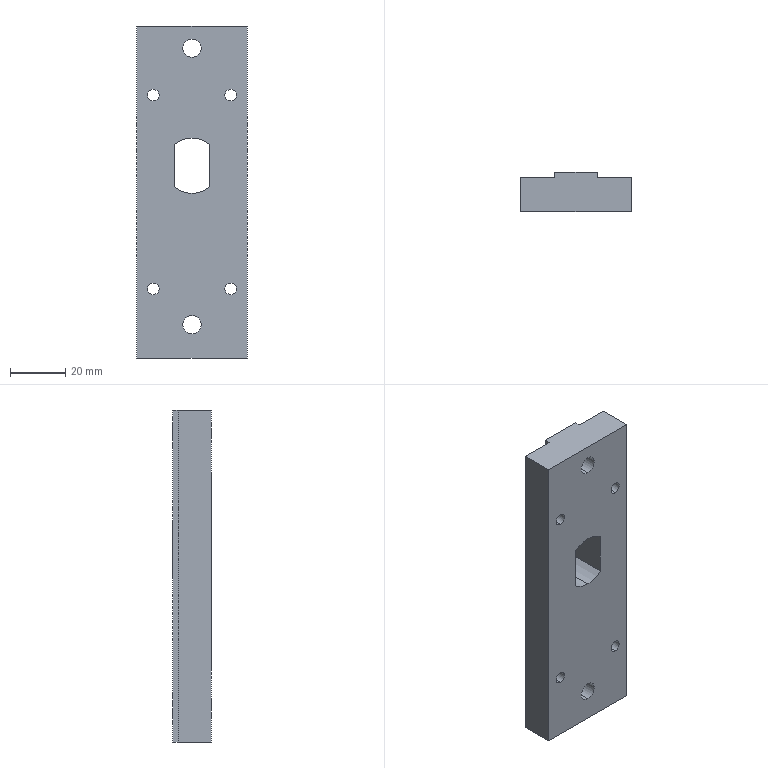Part | STEP file | magnetizing track | 1 solid | 33 faces | box 40 x 14 x 120 mm | volume 55579 mm3 | cylinder 19 | plane 14 | commonest cylinder face diameters 4.2 x8 6.6 x4 11 x4 20 x3